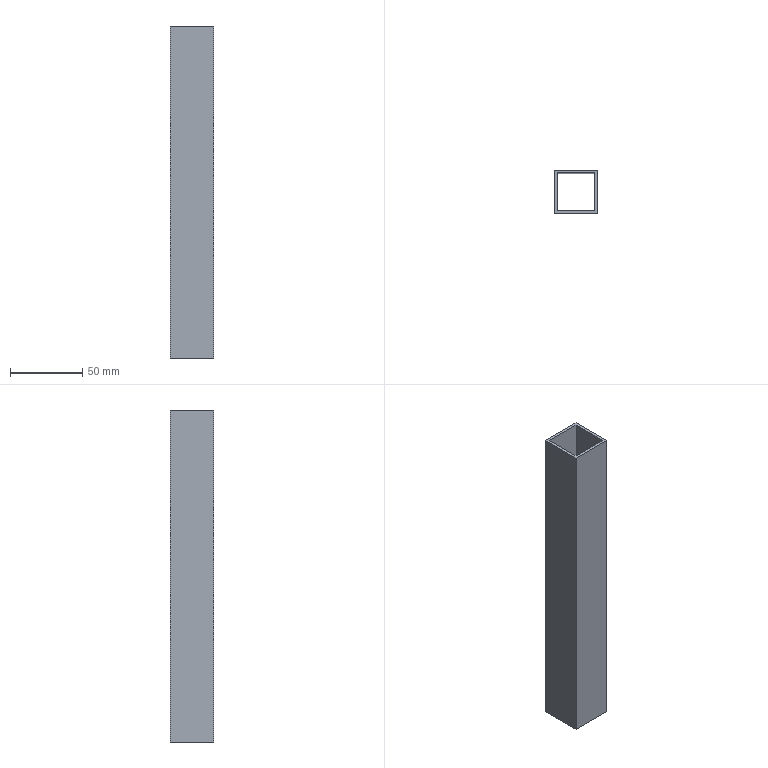Part | SolidWorks | features Extrusion 1 | 1 solid | 10 faces | box 30 x 30 x 230 mm | volume 51520 mm3 | plane 10
STEP:
#1=CARTESIAN_POINT('',(-15.,15.,115.));
#2=VERTEX_POINT('',#1);
#3=CARTESIAN_POINT('',(-15.,-15.,115.));
#4=VERTEX_POINT('',#3);
#5=CARTESIAN_POINT('',(-15.,-15.,115.));
#6=DIRECTION('',(0.,-1.,0.));
#7=VECTOR('',#6,1000.);
#8=LINE('',#5,#7);
#9=EDGE_CURVE('',#2,#4,#8,.T.);
#10=ORIENTED_EDGE('',*,*,#9,.T.);
#11=CARTESIAN_POINT('',(15.,-15.,115.));
#12=VERTEX_POINT('',#11);
#13=CARTESIAN_POINT('',(15.,-15.,115.));
#14=DIRECTION('',(1.,0.,0.));
#15=VECTOR('',#14,1000.);
#16=LINE('',#13,#15);
#17=EDGE_CURVE('',#4,#12,#16,.T.);
#18=ORIENTED_EDGE('',*,*,#17,.T.);
#19=CARTESIAN_POINT('',(15.,15.,115.));
#20=VERTEX_POINT('',#19);
#21=CARTESIAN_POINT('',(15.,-15.,115.));
#22=DIRECTION('',(0.,1.,0.));
#23=VECTOR('',#22,1000.);
#24=LINE('',#21,#23);
#25=EDGE_CURVE('',#12,#20,#24,.T.);
#26=ORIENTED_EDGE('',*,*,#25,.T.);
#27=CARTESIAN_POINT('',(15.,15.,115.));
#28=DIRECTION('',(-1.,0.,0.));
#29=VECTOR('',#28,1000.);
#30=LINE('',#27,#29);
#31=EDGE_CURVE('',#20,#2,#30,.T.);
#32=ORIENTED_EDGE('',*,*,#31,.T.);
#33=EDGE_LOOP('',(#10,#18,#26,#32));
#34=FACE_OUTER_BOUND('',#33,.T.);
#35=CARTESIAN_POINT('',(13.,-13.,115.));
#36=VERTEX_POINT('',#35);
#37=CARTESIAN_POINT('',(13.,13.,115.));
#38=VERTEX_POINT('',#37);
#39=CARTESIAN_POINT('',(13.,-13.,115.));
#40=DIRECTION('',(0.,1.,0.));
#41=VECTOR('',#40,1000.);
#42=LINE('',#39,#41);
#43=EDGE_CURVE('',#36,#38,#42,.T.);
#44=ORIENTED_EDGE('',*,*,#43,.F.);
#45=CARTESIAN_POINT('',(-13.,-13.,115.));
#46=VERTEX_POINT('',#45);
#47=CARTESIAN_POINT('',(13.,-13.,115.));
#48=DIRECTION('',(1.,0.,0.));
#49=VECTOR('',#48,1000.);
#50=LINE('',#47,#49);
#51=EDGE_CURVE('',#46,#36,#50,.T.);
#52=ORIENTED_EDGE('',*,*,#51,.F.);
#53=CARTESIAN_POINT('',(-13.,13.,115.));
#54=VERTEX_POINT('',#53);
#55=CARTESIAN_POINT('',(-13.,-13.,115.));
#56=DIRECTION('',(0.,-1.,0.));
#57=VECTOR('',#56,1000.);
#58=LINE('',#55,#57);
#59=EDGE_CURVE('',#54,#46,#58,.T.);
#60=ORIENTED_EDGE('',*,*,#59,.F.);
#61=CARTESIAN_POINT('',(13.,13.,115.));
#62=DIRECTION('',(-1.,0.,0.));
#63=VECTOR('',#62,1000.);
#64=LINE('',#61,#63);
#65=EDGE_CURVE('',#38,#54,#64,.T.);
#66=ORIENTED_EDGE('',*,*,#65,.F.);
#67=EDGE_LOOP('',(#44,#52,#60,#66));
#68=FACE_BOUND('',#67,.T.);
#69=CARTESIAN_POINT('',(0.,0.,115.));
#70=DIRECTION('',(0.,0.,1.));
#71=DIRECTION('',(1.,0.,0.));
#72=AXIS2_PLACEMENT_3D('',#69,#70,#71);
#73=PLANE('',#72);
#74=ADVANCED_FACE('',(#34,#68),#73,.T.);
#75=CARTESIAN_POINT('',(-15.,15.,-115.));
#76=VERTEX_POINT('',#75);
#77=CARTESIAN_POINT('',(-15.,-15.,-115.));
#78=VERTEX_POINT('',#77);
#79=CARTESIAN_POINT('',(-15.,-15.,-115.));
#80=DIRECTION('',(0.,-1.,0.));
#81=VECTOR('',#80,1000.);
#82=LINE('',#79,#81);
#83=EDGE_CURVE('',#76,#78,#82,.T.);
#84=ORIENTED_EDGE('',*,*,#83,.F.);
#85=CARTESIAN_POINT('',(15.,15.,-115.));
#86=VERTEX_POINT('',#85);
#87=CARTESIAN_POINT('',(15.,15.,-115.));
#88=DIRECTION('',(-1.,0.,0.));
#89=VECTOR('',#88,1000.);
#90=LINE('',#87,#89);
#91=EDGE_CURVE('',#86,#76,#90,.T.);
#92=ORIENTED_EDGE('',*,*,#91,.F.);
#93=CARTESIAN_POINT('',(15.,-15.,-115.));
#94=VERTEX_POINT('',#93);
#95=CARTESIAN_POINT('',(15.,-15.,-115.));
#96=DIRECTION('',(0.,1.,0.));
#97=VECTOR('',#96,1000.);
#98=LINE('',#95,#97);
#99=EDGE_CURVE('',#94,#86,#98,.T.);
#100=ORIENTED_EDGE('',*,*,#99,.F.);
#101=CARTESIAN_POINT('',(15.,-15.,-115.));
#102=DIRECTION('',(1.,0.,0.));
#103=VECTOR('',#102,1000.);
#104=LINE('',#101,#103);
#105=EDGE_CURVE('',#78,#94,#104,.T.);
#106=ORIENTED_EDGE('',*,*,#105,.F.);
#107=EDGE_LOOP('',(#84,#92,#100,#106));
#108=FACE_OUTER_BOUND('',#107,.T.);
#109=CARTESIAN_POINT('',(-13.,-13.,-115.));
#110=VERTEX_POINT('',#109);
#111=CARTESIAN_POINT('',(13.,-13.,-115.));
#112=VERTEX_POINT('',#111);
#113=CARTESIAN_POINT('',(13.,-13.,-115.));
#114=DIRECTION('',(1.,0.,0.));
#115=VECTOR('',#114,1000.);
#116=LINE('',#113,#115);
#117=EDGE_CURVE('',#110,#112,#116,.T.);
#118=ORIENTED_EDGE('',*,*,#117,.T.);
#119=CARTESIAN_POINT('',(13.,13.,-115.));
#120=VERTEX_POINT('',#119);
#121=CARTESIAN_POINT('',(13.,-13.,-115.));
#122=DIRECTION('',(0.,1.,0.));
#123=VECTOR('',#122,1000.);
#124=LINE('',#121,#123);
#125=EDGE_CURVE('',#112,#120,#124,.T.);
#126=ORIENTED_EDGE('',*,*,#125,.T.);
#127=CARTESIAN_POINT('',(-13.,13.,-115.));
#128=VERTEX_POINT('',#127);
#129=CARTESIAN_POINT('',(13.,13.,-115.));
#130=DIRECTION('',(-1.,0.,0.));
#131=VECTOR('',#130,1000.);
#132=LINE('',#129,#131);
#133=EDGE_CURVE('',#120,#128,#132,.T.);
#134=ORIENTED_EDGE('',*,*,#133,.T.);
#135=CARTESIAN_POINT('',(-13.,-13.,-115.));
#136=DIRECTION('',(0.,-1.,0.));
#137=VECTOR('',#136,1000.);
#138=LINE('',#135,#137);
#139=EDGE_CURVE('',#128,#110,#138,.T.);
#140=ORIENTED_EDGE('',*,*,#139,.T.);
#141=EDGE_LOOP('',(#118,#126,#134,#140));
#142=FACE_BOUND('',#141,.T.);
#143=CARTESIAN_POINT('',(0.,0.,-115.));
#144=DIRECTION('',(0.,0.,1.));
#145=DIRECTION('',(1.,0.,0.));
#146=AXIS2_PLACEMENT_3D('',#143,#144,#145);
#147=PLANE('',#146);
#148=ADVANCED_FACE('',(#108,#142),#147,.F.);
#149=ORIENTED_EDGE('',*,*,#83,.T.);
#150=CARTESIAN_POINT('',(-15.,-15.,115.));
#151=DIRECTION('',(0.,0.,-1.));
#152=VECTOR('',#151,1000.);
#153=LINE('',#150,#152);
#154=EDGE_CURVE('',#4,#78,#153,.T.);
#155=ORIENTED_EDGE('',*,*,#154,.F.);
#156=ORIENTED_EDGE('',*,*,#9,.F.);
#157=CARTESIAN_POINT('',(-15.,15.,115.));
#158=DIRECTION('',(0.,0.,-1.));
#159=VECTOR('',#158,1000.);
#160=LINE('',#157,#159);
#161=EDGE_CURVE('',#2,#76,#160,.T.);
#162=ORIENTED_EDGE('',*,*,#161,.T.);
#163=EDGE_LOOP('',(#149,#155,#156,#162));
#164=FACE_OUTER_BOUND('',#163,.T.);
#165=CARTESIAN_POINT('',(-15.,-15.,115.));
#166=DIRECTION('',(1.,0.,0.));
#167=DIRECTION('',(0.,1.,0.));
#168=AXIS2_PLACEMENT_3D('',#165,#166,#167);
#169=PLANE('',#168);
#170=ADVANCED_FACE('',(#164),#169,.F.);
#171=ORIENTED_EDGE('',*,*,#105,.T.);
#172=CARTESIAN_POINT('',(15.,-15.,115.));
#173=DIRECTION('',(0.,0.,-1.));
#174=VECTOR('',#173,1000.);
#175=LINE('',#172,#174);
#176=EDGE_CURVE('',#12,#94,#175,.T.);
#177=ORIENTED_EDGE('',*,*,#176,.F.);
#178=ORIENTED_EDGE('',*,*,#17,.F.);
#179=ORIENTED_EDGE('',*,*,#154,.T.);
#180=EDGE_LOOP('',(#171,#177,#178,#179));
#181=FACE_OUTER_BOUND('',#180,.T.);
#182=CARTESIAN_POINT('',(15.,-15.,115.));
#183=DIRECTION('',(0.,1.,0.));
#184=DIRECTION('',(-1.,0.,0.));
#185=AXIS2_PLACEMENT_3D('',#182,#183,#184);
#186=PLANE('',#185);
#187=ADVANCED_FACE('',(#181),#186,.F.);
#188=ORIENTED_EDGE('',*,*,#99,.T.);
#189=CARTESIAN_POINT('',(15.,15.,115.));
#190=DIRECTION('',(0.,0.,-1.));
#191=VECTOR('',#190,1000.);
#192=LINE('',#189,#191);
#193=EDGE_CURVE('',#20,#86,#192,.T.);
#194=ORIENTED_EDGE('',*,*,#193,.F.);
#195=ORIENTED_EDGE('',*,*,#25,.F.);
#196=ORIENTED_EDGE('',*,*,#176,.T.);
#197=EDGE_LOOP('',(#188,#194,#195,#196));
#198=FACE_OUTER_BOUND('',#197,.T.);
#199=CARTESIAN_POINT('',(15.,-15.,115.));
#200=DIRECTION('',(-1.,0.,0.));
#201=DIRECTION('',(0.,0.,1.));
#202=AXIS2_PLACEMENT_3D('',#199,#200,#201);
#203=PLANE('',#202);
#204=ADVANCED_FACE('',(#198),#203,.F.);
#205=ORIENTED_EDGE('',*,*,#91,.T.);
#206=ORIENTED_EDGE('',*,*,#161,.F.);
#207=ORIENTED_EDGE('',*,*,#31,.F.);
#208=ORIENTED_EDGE('',*,*,#193,.T.);
#209=EDGE_LOOP('',(#205,#206,#207,#208));
#210=FACE_OUTER_BOUND('',#209,.T.);
#211=CARTESIAN_POINT('',(15.,15.,115.));
#212=DIRECTION('',(0.,-1.,0.));
#213=DIRECTION('',(0.,0.,-1.));
#214=AXIS2_PLACEMENT_3D('',#211,#212,#213);
#215=PLANE('',#214);
#216=ADVANCED_FACE('',(#210),#215,.F.);
#217=ORIENTED_EDGE('',*,*,#117,.F.);
#218=CARTESIAN_POINT('',(-13.,-13.,115.));
#219=DIRECTION('',(0.,0.,-1.));
#220=VECTOR('',#219,1000.);
#221=LINE('',#218,#220);
#222=EDGE_CURVE('',#46,#110,#221,.T.);
#223=ORIENTED_EDGE('',*,*,#222,.F.);
#224=ORIENTED_EDGE('',*,*,#51,.T.);
#225=CARTESIAN_POINT('',(13.,-13.,115.));
#226=DIRECTION('',(0.,0.,-1.));
#227=VECTOR('',#226,1000.);
#228=LINE('',#225,#227);
#229=EDGE_CURVE('',#36,#112,#228,.T.);
#230=ORIENTED_EDGE('',*,*,#229,.T.);
#231=EDGE_LOOP('',(#217,#223,#224,#230));
#232=FACE_OUTER_BOUND('',#231,.T.);
#233=CARTESIAN_POINT('',(13.,-13.,115.));
#234=DIRECTION('',(0.,1.,0.));
#235=DIRECTION('',(0.,0.,1.));
#236=AXIS2_PLACEMENT_3D('',#233,#234,#235);
#237=PLANE('',#236);
#238=ADVANCED_FACE('',(#232),#237,.T.);
#239=ORIENTED_EDGE('',*,*,#125,.F.);
#240=ORIENTED_EDGE('',*,*,#229,.F.);
#241=ORIENTED_EDGE('',*,*,#43,.T.);
#242=CARTESIAN_POINT('',(13.,13.,115.));
#243=DIRECTION('',(0.,0.,-1.));
#244=VECTOR('',#243,1000.);
#245=LINE('',#242,#244);
#246=EDGE_CURVE('',#38,#120,#245,.T.);
#247=ORIENTED_EDGE('',*,*,#246,.T.);
#248=EDGE_LOOP('',(#239,#240,#241,#247));
#249=FACE_OUTER_BOUND('',#248,.T.);
#250=CARTESIAN_POINT('',(13.,-13.,115.));
#251=DIRECTION('',(-1.,0.,0.));
#252=DIRECTION('',(0.,0.,1.));
#253=AXIS2_PLACEMENT_3D('',#250,#251,#252);
#254=PLANE('',#253);
#255=ADVANCED_FACE('',(#249),#254,.T.);
#256=ORIENTED_EDGE('',*,*,#133,.F.);
#257=ORIENTED_EDGE('',*,*,#246,.F.);
#258=ORIENTED_EDGE('',*,*,#65,.T.);
#259=CARTESIAN_POINT('',(-13.,13.,115.));
#260=DIRECTION('',(0.,0.,-1.));
#261=VECTOR('',#260,1000.);
#262=LINE('',#259,#261);
#263=EDGE_CURVE('',#54,#128,#262,.T.);
#264=ORIENTED_EDGE('',*,*,#263,.T.);
#265=EDGE_LOOP('',(#256,#257,#258,#264));
#266=FACE_OUTER_BOUND('',#265,.T.);
#267=CARTESIAN_POINT('',(13.,13.,115.));
#268=DIRECTION('',(0.,-1.,0.));
#269=DIRECTION('',(0.,0.,-1.));
#270=AXIS2_PLACEMENT_3D('',#267,#268,#269);
#271=PLANE('',#270);
#272=ADVANCED_FACE('',(#266),#271,.T.);
#273=ORIENTED_EDGE('',*,*,#139,.F.);
#274=ORIENTED_EDGE('',*,*,#263,.F.);
#275=ORIENTED_EDGE('',*,*,#59,.T.);
#276=ORIENTED_EDGE('',*,*,#222,.T.);
#277=EDGE_LOOP('',(#273,#274,#275,#276));
#278=FACE_OUTER_BOUND('',#277,.T.);
#279=CARTESIAN_POINT('',(-13.,-13.,115.));
#280=DIRECTION('',(1.,0.,0.));
#281=DIRECTION('',(0.,0.,-1.));
#282=AXIS2_PLACEMENT_3D('',#279,#280,#281);
#283=PLANE('',#282);
#284=ADVANCED_FACE('',(#278),#283,.T.);
#285=CLOSED_SHELL('',(#74,#148,#170,#187,#204,#216,#238,#255,#272,#284));
#286=MANIFOLD_SOLID_BREP('',#285);
#287=CARTESIAN_POINT('',(0.,0.,0.));
#288=DIRECTION('',(0.,0.,1.));
#289=DIRECTION('',(1.,0.,0.));
#290=AXIS2_PLACEMENT_3D('',#287,#288,#289);
#291=(LENGTH_UNIT()NAMED_UNIT(*)SI_UNIT(.MILLI.,.METRE.));
#292=UNCERTAINTY_MEASURE_WITH_UNIT(LENGTH_MEASURE(0.00001),#291,'','');
#293=(NAMED_UNIT(*)PLANE_ANGLE_UNIT()SI_UNIT($,.RADIAN.));
#294=(NAMED_UNIT(*)SI_UNIT($,.STERADIAN.)SOLID_ANGLE_UNIT());
#295=(GEOMETRIC_REPRESENTATION_CONTEXT(3)GLOBAL_UNCERTAINTY_ASSIGNED_CONTEXT((#292))GLOBAL_UNIT_ASSIGNED_CONTEXT((#291,#293,#294))REPRESENTATION_CONTEXT('',''));
#296=ADVANCED_BREP_SHAPE_REPRESENTATION('',(#286,#290),#295);